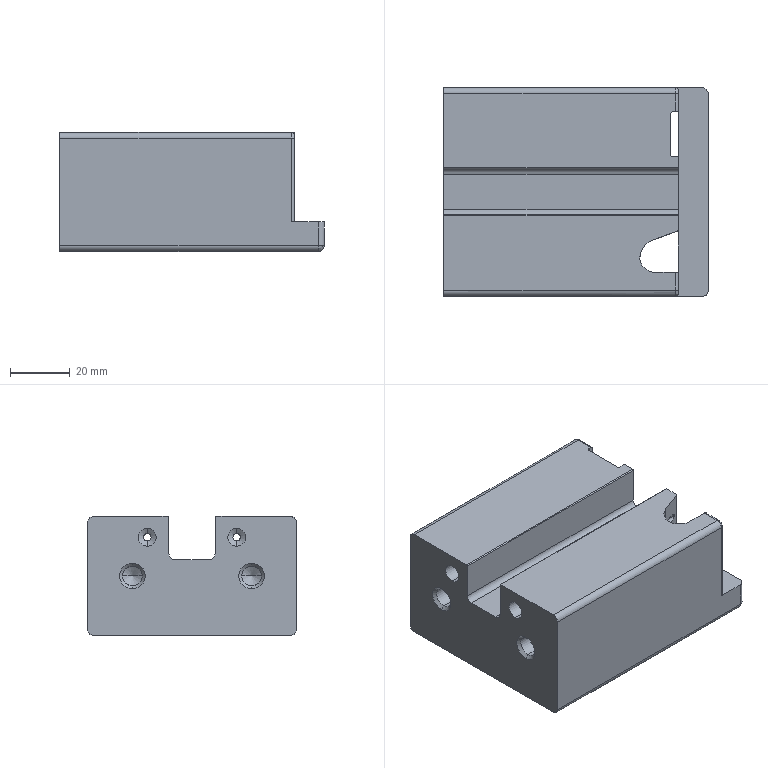Part | STEP file | LUOI CAT KHONG LOGO | 1 solid | 77 faces | box 88.8 x 70 x 40 mm | volume 196221 mm3 | cylinder 35 | plane 21 | cone 16 | spline 5 | commonest cylinder face diameters 4 x9 6.647 x6 2 x5 2.5 x4 6 x4 1 x3